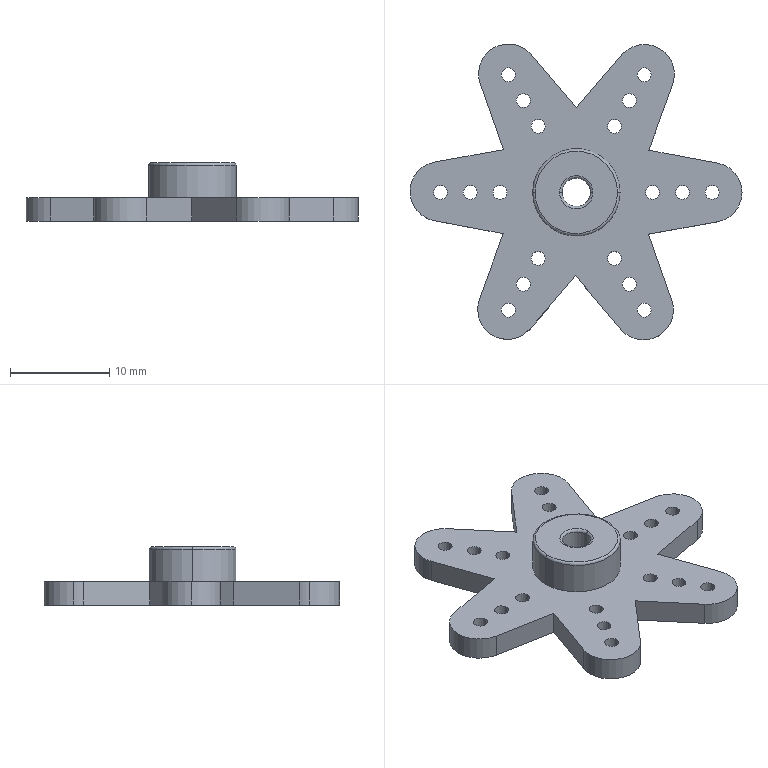Part | SolidWorks | features ICE 4, Extrusion 1, Fillet 1 | 1 solid | 77 faces | box 33.41 x 29.789 x 5.85 mm | volume 1360 mm3 | cylinder 55 | plane 18 | torus 4 | commonest cylinder face diameters 1.4 x36 6 x11 2.85 x2 7 x2 8.5 x2 8.8 x2